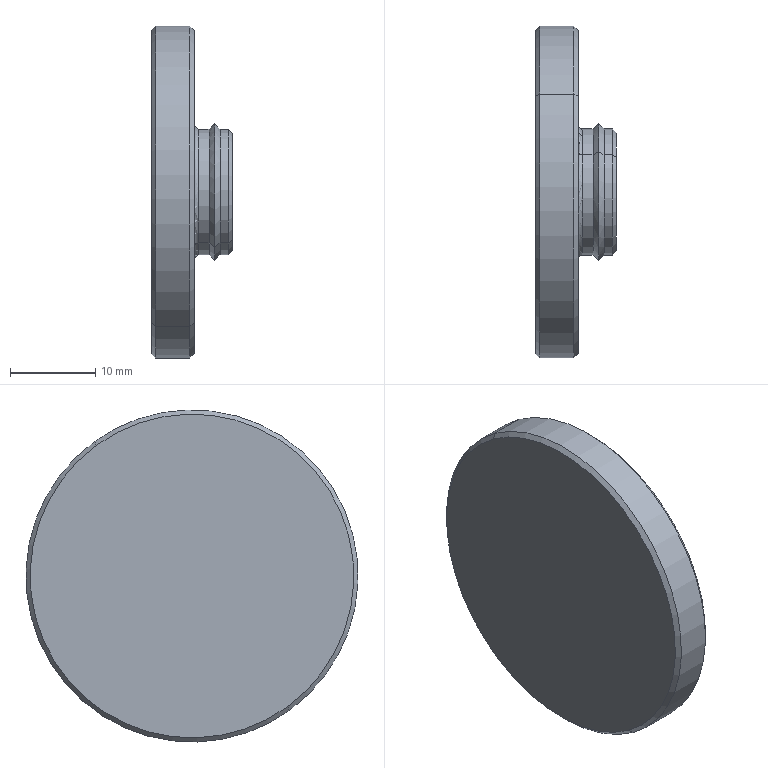Part | STEP file | Disc Pad | 1 solid | 21 faces | box 9.5 x 39 x 39 mm | volume 6734 mm3 | cone 10 | cylinder 6 | plane 3 | torus 2 | commonest cylinder face diameters 14.8 x4 39 x2